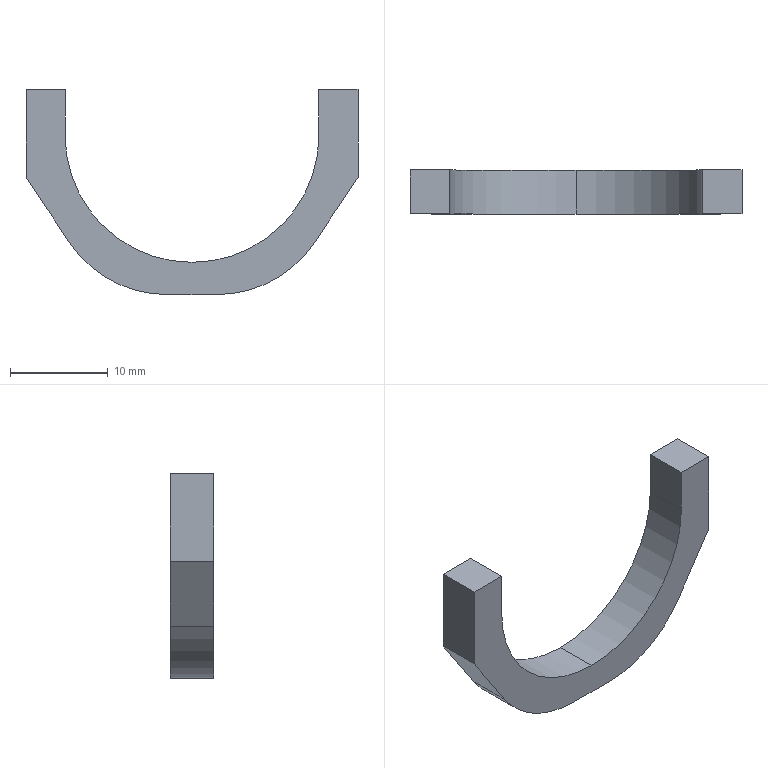Part | SolidWorks | features FlatPattern 1, SMBaseFlange 1, SheetMetal 1 | 1 solid | 15 faces | box 34 x 4.5 x 21 mm | volume 979.762 mm3 | plane 11 | cylinder 4 | commonest cylinder face diameters 24 x2 26 x2
STEP:
#1=CARTESIAN_POINT('',(0.,4.5,3.3));
#2=VERTEX_POINT('',#1);
#3=CARTESIAN_POINT('',(13.,4.5,16.3));
#4=VERTEX_POINT('',#3);
#5=CARTESIAN_POINT('',(0.,4.5,16.3));
#6=DIRECTION('',(0.,-1.,0.));
#7=DIRECTION('',(0.,0.,1.));
#8=AXIS2_PLACEMENT_3D('',#5,#6,#7);
#9=CIRCLE('',#8,13.);
#10=EDGE_CURVE('',#2,#4,#9,.T.);
#11=ORIENTED_EDGE('',*,*,#10,.F.);
#12=CARTESIAN_POINT('',(0.,0.,3.3));
#13=VERTEX_POINT('',#12);
#14=CARTESIAN_POINT('',(0.,4.5,3.3));
#15=DIRECTION('',(0.,-1.,0.));
#16=VECTOR('',#15,1000.);
#17=LINE('',#14,#16);
#18=EDGE_CURVE('',#2,#13,#17,.T.);
#19=ORIENTED_EDGE('',*,*,#18,.T.);
#20=CARTESIAN_POINT('',(13.,0.,16.3));
#21=VERTEX_POINT('',#20);
#22=CARTESIAN_POINT('',(0.,0.,16.3));
#23=DIRECTION('',(0.,-1.,0.));
#24=DIRECTION('',(0.,0.,1.));
#25=AXIS2_PLACEMENT_3D('',#22,#23,#24);
#26=CIRCLE('',#25,13.);
#27=EDGE_CURVE('',#13,#21,#26,.T.);
#28=ORIENTED_EDGE('',*,*,#27,.T.);
#29=CARTESIAN_POINT('',(13.,4.5,16.3));
#30=DIRECTION('',(0.,-1.,0.));
#31=VECTOR('',#30,1000.);
#32=LINE('',#29,#31);
#33=EDGE_CURVE('',#4,#21,#32,.T.);
#34=ORIENTED_EDGE('',*,*,#33,.F.);
#35=EDGE_LOOP('',(#11,#19,#28,#34));
#36=FACE_OUTER_BOUND('',#35,.T.);
#37=CARTESIAN_POINT('',(0.,4.5,16.3));
#38=DIRECTION('',(0.,-1.,0.));
#39=DIRECTION('',(0.,0.,-1.));
#40=AXIS2_PLACEMENT_3D('',#37,#38,#39);
#41=CYLINDRICAL_SURFACE('',#40,13.);
#42=ADVANCED_FACE('',(#36),#41,.F.);
#43=CARTESIAN_POINT('',(-12.562,0.,5.344));
#44=VERTEX_POINT('',#43);
#45=CARTESIAN_POINT('',(-17.,0.,12.));
#46=VERTEX_POINT('',#45);
#47=CARTESIAN_POINT('',(-12.562,0.,5.344));
#48=DIRECTION('',(-0.5547,0.,0.8321));
#49=VECTOR('',#48,1000.);
#50=LINE('',#47,#49);
#51=EDGE_CURVE('',#44,#46,#50,.T.);
#52=ORIENTED_EDGE('',*,*,#51,.T.);
#53=CARTESIAN_POINT('',(-17.,4.5,12.));
#54=VERTEX_POINT('',#53);
#55=CARTESIAN_POINT('',(-17.,4.5,12.));
#56=DIRECTION('',(0.,-1.,0.));
#57=VECTOR('',#56,1000.);
#58=LINE('',#55,#57);
#59=EDGE_CURVE('',#54,#46,#58,.T.);
#60=ORIENTED_EDGE('',*,*,#59,.F.);
#61=CARTESIAN_POINT('',(-12.562,4.5,5.344));
#62=VERTEX_POINT('',#61);
#63=CARTESIAN_POINT('',(-12.562,4.5,5.344));
#64=DIRECTION('',(-0.5547,0.,0.8321));
#65=VECTOR('',#64,1000.);
#66=LINE('',#63,#65);
#67=EDGE_CURVE('',#62,#54,#66,.T.);
#68=ORIENTED_EDGE('',*,*,#67,.F.);
#69=CARTESIAN_POINT('',(-12.562,4.5,5.344));
#70=DIRECTION('',(0.,-1.,0.));
#71=VECTOR('',#70,1000.);
#72=LINE('',#69,#71);
#73=EDGE_CURVE('',#62,#44,#72,.T.);
#74=ORIENTED_EDGE('',*,*,#73,.T.);
#75=EDGE_LOOP('',(#52,#60,#68,#74));
#76=FACE_OUTER_BOUND('',#75,.T.);
#77=CARTESIAN_POINT('',(-12.562,4.5,5.344));
#78=DIRECTION('',(0.8321,0.,0.5547));
#79=DIRECTION('',(0.5547,0.,-0.8321));
#80=AXIS2_PLACEMENT_3D('',#77,#78,#79);
#81=PLANE('',#80);
#82=ADVANCED_FACE('',(#76),#81,.F.);
#83=CARTESIAN_POINT('',(-17.,0.,21.));
#84=VERTEX_POINT('',#83);
#85=CARTESIAN_POINT('',(-17.,0.,12.));
#86=DIRECTION('',(0.,0.,1.));
#87=VECTOR('',#86,1000.);
#88=LINE('',#85,#87);
#89=EDGE_CURVE('',#46,#84,#88,.T.);
#90=ORIENTED_EDGE('',*,*,#89,.T.);
#91=CARTESIAN_POINT('',(-17.,4.5,21.));
#92=VERTEX_POINT('',#91);
#93=CARTESIAN_POINT('',(-17.,4.5,21.));
#94=DIRECTION('',(0.,-1.,0.));
#95=VECTOR('',#94,1000.);
#96=LINE('',#93,#95);
#97=EDGE_CURVE('',#92,#84,#96,.T.);
#98=ORIENTED_EDGE('',*,*,#97,.F.);
#99=CARTESIAN_POINT('',(-17.,4.5,12.));
#100=DIRECTION('',(0.,0.,1.));
#101=VECTOR('',#100,1000.);
#102=LINE('',#99,#101);
#103=EDGE_CURVE('',#54,#92,#102,.T.);
#104=ORIENTED_EDGE('',*,*,#103,.F.);
#105=ORIENTED_EDGE('',*,*,#59,.T.);
#106=EDGE_LOOP('',(#90,#98,#104,#105));
#107=FACE_OUTER_BOUND('',#106,.T.);
#108=CARTESIAN_POINT('',(-17.,4.5,12.));
#109=DIRECTION('',(1.,0.,0.));
#110=DIRECTION('',(0.,0.,-1.));
#111=AXIS2_PLACEMENT_3D('',#108,#109,#110);
#112=PLANE('',#111);
#113=ADVANCED_FACE('',(#107),#112,.F.);
#114=CARTESIAN_POINT('',(-13.,0.,21.));
#115=VERTEX_POINT('',#114);
#116=CARTESIAN_POINT('',(-13.,0.,21.));
#117=DIRECTION('',(1.,0.,0.));
#118=VECTOR('',#117,1000.);
#119=LINE('',#116,#118);
#120=EDGE_CURVE('',#84,#115,#119,.T.);
#121=ORIENTED_EDGE('',*,*,#120,.T.);
#122=CARTESIAN_POINT('',(-13.,4.5,21.));
#123=VERTEX_POINT('',#122);
#124=CARTESIAN_POINT('',(-13.,4.5,21.));
#125=DIRECTION('',(0.,-1.,0.));
#126=VECTOR('',#125,1000.);
#127=LINE('',#124,#126);
#128=EDGE_CURVE('',#123,#115,#127,.T.);
#129=ORIENTED_EDGE('',*,*,#128,.F.);
#130=CARTESIAN_POINT('',(-13.,4.5,21.));
#131=DIRECTION('',(1.,0.,0.));
#132=VECTOR('',#131,1000.);
#133=LINE('',#130,#132);
#134=EDGE_CURVE('',#92,#123,#133,.T.);
#135=ORIENTED_EDGE('',*,*,#134,.F.);
#136=ORIENTED_EDGE('',*,*,#97,.T.);
#137=EDGE_LOOP('',(#121,#129,#135,#136));
#138=FACE_OUTER_BOUND('',#137,.T.);
#139=CARTESIAN_POINT('',(-13.,4.5,21.));
#140=DIRECTION('',(0.,0.,-1.));
#141=DIRECTION('',(-1.,0.,0.));
#142=AXIS2_PLACEMENT_3D('',#139,#140,#141);
#143=PLANE('',#142);
#144=ADVANCED_FACE('',(#138),#143,.F.);
#145=CARTESIAN_POINT('',(-13.,0.,16.3));
#146=VERTEX_POINT('',#145);
#147=CARTESIAN_POINT('',(-13.,0.,16.3));
#148=DIRECTION('',(0.,0.,-1.));
#149=VECTOR('',#148,1000.);
#150=LINE('',#147,#149);
#151=EDGE_CURVE('',#115,#146,#150,.T.);
#152=ORIENTED_EDGE('',*,*,#151,.T.);
#153=CARTESIAN_POINT('',(-13.,4.5,16.3));
#154=VERTEX_POINT('',#153);
#155=CARTESIAN_POINT('',(-13.,4.5,16.3));
#156=DIRECTION('',(0.,-1.,0.));
#157=VECTOR('',#156,1000.);
#158=LINE('',#155,#157);
#159=EDGE_CURVE('',#154,#146,#158,.T.);
#160=ORIENTED_EDGE('',*,*,#159,.F.);
#161=CARTESIAN_POINT('',(-13.,4.5,16.3));
#162=DIRECTION('',(0.,0.,-1.));
#163=VECTOR('',#162,1000.);
#164=LINE('',#161,#163);
#165=EDGE_CURVE('',#123,#154,#164,.T.);
#166=ORIENTED_EDGE('',*,*,#165,.F.);
#167=ORIENTED_EDGE('',*,*,#128,.T.);
#168=EDGE_LOOP('',(#152,#160,#166,#167));
#169=FACE_OUTER_BOUND('',#168,.T.);
#170=CARTESIAN_POINT('',(-13.,4.5,16.3));
#171=DIRECTION('',(-1.,0.,0.));
#172=DIRECTION('',(0.,0.,1.));
#173=AXIS2_PLACEMENT_3D('',#170,#171,#172);
#174=PLANE('',#173);
#175=ADVANCED_FACE('',(#169),#174,.F.);
#176=ORIENTED_EDGE('',*,*,#18,.F.);
#177=CARTESIAN_POINT('',(0.,4.5,16.3));
#178=DIRECTION('',(0.,-1.,0.));
#179=DIRECTION('',(0.,0.,1.));
#180=AXIS2_PLACEMENT_3D('',#177,#178,#179);
#181=CIRCLE('',#180,13.);
#182=EDGE_CURVE('',#154,#2,#181,.T.);
#183=ORIENTED_EDGE('',*,*,#182,.F.);
#184=ORIENTED_EDGE('',*,*,#159,.T.);
#185=CARTESIAN_POINT('',(0.,0.,16.3));
#186=DIRECTION('',(0.,-1.,0.));
#187=DIRECTION('',(0.,0.,1.));
#188=AXIS2_PLACEMENT_3D('',#185,#186,#187);
#189=CIRCLE('',#188,13.);
#190=EDGE_CURVE('',#146,#13,#189,.T.);
#191=ORIENTED_EDGE('',*,*,#190,.T.);
#192=EDGE_LOOP('',(#176,#183,#184,#191));
#193=FACE_OUTER_BOUND('',#192,.T.);
#194=CARTESIAN_POINT('',(0.,4.5,16.3));
#195=DIRECTION('',(0.,-1.,0.));
#196=DIRECTION('',(0.,0.,-1.));
#197=AXIS2_PLACEMENT_3D('',#194,#195,#196);
#198=CYLINDRICAL_SURFACE('',#197,13.);
#199=ADVANCED_FACE('',(#193),#198,.F.);
#200=CARTESIAN_POINT('',(13.,0.,21.));
#201=VERTEX_POINT('',#200);
#202=CARTESIAN_POINT('',(13.,0.,16.3));
#203=DIRECTION('',(0.,0.,1.));
#204=VECTOR('',#203,1000.);
#205=LINE('',#202,#204);
#206=EDGE_CURVE('',#21,#201,#205,.T.);
#207=ORIENTED_EDGE('',*,*,#206,.T.);
#208=CARTESIAN_POINT('',(13.,4.5,21.));
#209=VERTEX_POINT('',#208);
#210=CARTESIAN_POINT('',(13.,4.5,21.));
#211=DIRECTION('',(0.,-1.,0.));
#212=VECTOR('',#211,1000.);
#213=LINE('',#210,#212);
#214=EDGE_CURVE('',#209,#201,#213,.T.);
#215=ORIENTED_EDGE('',*,*,#214,.F.);
#216=CARTESIAN_POINT('',(13.,4.5,16.3));
#217=DIRECTION('',(0.,0.,1.));
#218=VECTOR('',#217,1000.);
#219=LINE('',#216,#218);
#220=EDGE_CURVE('',#4,#209,#219,.T.);
#221=ORIENTED_EDGE('',*,*,#220,.F.);
#222=ORIENTED_EDGE('',*,*,#33,.T.);
#223=EDGE_LOOP('',(#207,#215,#221,#222));
#224=FACE_OUTER_BOUND('',#223,.T.);
#225=CARTESIAN_POINT('',(13.,4.5,16.3));
#226=DIRECTION('',(1.,0.,0.));
#227=DIRECTION('',(0.,0.,-1.));
#228=AXIS2_PLACEMENT_3D('',#225,#226,#227);
#229=PLANE('',#228);
#230=ADVANCED_FACE('',(#224),#229,.F.);
#231=CARTESIAN_POINT('',(17.,0.,21.));
#232=VERTEX_POINT('',#231);
#233=CARTESIAN_POINT('',(13.,0.,21.));
#234=DIRECTION('',(1.,0.,0.));
#235=VECTOR('',#234,1000.);
#236=LINE('',#233,#235);
#237=EDGE_CURVE('',#201,#232,#236,.T.);
#238=ORIENTED_EDGE('',*,*,#237,.T.);
#239=CARTESIAN_POINT('',(17.,4.5,21.));
#240=VERTEX_POINT('',#239);
#241=CARTESIAN_POINT('',(17.,4.5,21.));
#242=DIRECTION('',(0.,-1.,0.));
#243=VECTOR('',#242,1000.);
#244=LINE('',#241,#243);
#245=EDGE_CURVE('',#240,#232,#244,.T.);
#246=ORIENTED_EDGE('',*,*,#245,.F.);
#247=CARTESIAN_POINT('',(13.,4.5,21.));
#248=DIRECTION('',(1.,0.,0.));
#249=VECTOR('',#248,1000.);
#250=LINE('',#247,#249);
#251=EDGE_CURVE('',#209,#240,#250,.T.);
#252=ORIENTED_EDGE('',*,*,#251,.F.);
#253=ORIENTED_EDGE('',*,*,#214,.T.);
#254=EDGE_LOOP('',(#238,#246,#252,#253));
#255=FACE_OUTER_BOUND('',#254,.T.);
#256=CARTESIAN_POINT('',(13.,4.5,21.));
#257=DIRECTION('',(0.,0.,-1.));
#258=DIRECTION('',(-1.,0.,0.));
#259=AXIS2_PLACEMENT_3D('',#256,#257,#258);
#260=PLANE('',#259);
#261=ADVANCED_FACE('',(#255),#260,.F.);
#262=CARTESIAN_POINT('',(17.,0.,12.));
#263=VERTEX_POINT('',#262);
#264=CARTESIAN_POINT('',(17.,0.,12.));
#265=DIRECTION('',(0.,0.,-1.));
#266=VECTOR('',#265,1000.);
#267=LINE('',#264,#266);
#268=EDGE_CURVE('',#232,#263,#267,.T.);
#269=ORIENTED_EDGE('',*,*,#268,.T.);
#270=CARTESIAN_POINT('',(17.,4.5,12.));
#271=VERTEX_POINT('',#270);
#272=CARTESIAN_POINT('',(17.,4.5,12.));
#273=DIRECTION('',(0.,-1.,0.));
#274=VECTOR('',#273,1000.);
#275=LINE('',#272,#274);
#276=EDGE_CURVE('',#271,#263,#275,.T.);
#277=ORIENTED_EDGE('',*,*,#276,.F.);
#278=CARTESIAN_POINT('',(17.,4.5,12.));
#279=DIRECTION('',(0.,0.,-1.));
#280=VECTOR('',#279,1000.);
#281=LINE('',#278,#280);
#282=EDGE_CURVE('',#240,#271,#281,.T.);
#283=ORIENTED_EDGE('',*,*,#282,.F.);
#284=ORIENTED_EDGE('',*,*,#245,.T.);
#285=EDGE_LOOP('',(#269,#277,#283,#284));
#286=FACE_OUTER_BOUND('',#285,.T.);
#287=CARTESIAN_POINT('',(17.,4.5,12.));
#288=DIRECTION('',(-1.,0.,0.));
#289=DIRECTION('',(0.,0.,1.));
#290=AXIS2_PLACEMENT_3D('',#287,#288,#289);
#291=PLANE('',#290);
#292=ADVANCED_FACE('',(#286),#291,.F.);
#293=CARTESIAN_POINT('',(12.562,0.,5.344));
#294=VERTEX_POINT('',#293);
#295=CARTESIAN_POINT('',(12.562,0.,5.344));
#296=DIRECTION('',(-0.5547,0.,-0.8321));
#297=VECTOR('',#296,1000.);
#298=LINE('',#295,#297);
#299=EDGE_CURVE('',#263,#294,#298,.T.);
#300=ORIENTED_EDGE('',*,*,#299,.T.);
#301=CARTESIAN_POINT('',(12.562,4.5,5.344));
#302=VERTEX_POINT('',#301);
#303=CARTESIAN_POINT('',(12.562,4.5,5.344));
#304=DIRECTION('',(0.,-1.,0.));
#305=VECTOR('',#304,1000.);
#306=LINE('',#303,#305);
#307=EDGE_CURVE('',#302,#294,#306,.T.);
#308=ORIENTED_EDGE('',*,*,#307,.F.);
#309=CARTESIAN_POINT('',(12.562,4.5,5.344));
#310=DIRECTION('',(-0.5547,0.,-0.8321));
#311=VECTOR('',#310,1000.);
#312=LINE('',#309,#311);
#313=EDGE_CURVE('',#271,#302,#312,.T.);
#314=ORIENTED_EDGE('',*,*,#313,.F.);
#315=ORIENTED_EDGE('',*,*,#276,.T.);
#316=EDGE_LOOP('',(#300,#308,#314,#315));
#317=FACE_OUTER_BOUND('',#316,.T.);
#318=CARTESIAN_POINT('',(12.562,4.5,5.344));
#319=DIRECTION('',(-0.8321,0.,0.5547));
#320=DIRECTION('',(0.5547,0.,0.8321));
#321=AXIS2_PLACEMENT_3D('',#318,#319,#320);
#322=PLANE('',#321);
#323=ADVANCED_FACE('',(#317),#322,.F.);
#324=CARTESIAN_POINT('',(2.578,0.,0.));
#325=VERTEX_POINT('',#324);
#326=CARTESIAN_POINT('',(2.578,0.,12.));
#327=DIRECTION('',(0.,1.,0.));
#328=DIRECTION('',(0.,0.,-1.));
#329=AXIS2_PLACEMENT_3D('',#326,#327,#328);
#330=CIRCLE('',#329,12.);
#331=EDGE_CURVE('',#294,#325,#330,.T.);
#332=ORIENTED_EDGE('',*,*,#331,.T.);
#333=CARTESIAN_POINT('',(2.578,4.5,0.));
#334=VERTEX_POINT('',#333);
#335=CARTESIAN_POINT('',(2.578,4.5,0.));
#336=DIRECTION('',(0.,-1.,0.));
#337=VECTOR('',#336,1000.);
#338=LINE('',#335,#337);
#339=EDGE_CURVE('',#334,#325,#338,.T.);
#340=ORIENTED_EDGE('',*,*,#339,.F.);
#341=CARTESIAN_POINT('',(2.578,4.5,12.));
#342=DIRECTION('',(0.,1.,0.));
#343=DIRECTION('',(0.,0.,-1.));
#344=AXIS2_PLACEMENT_3D('',#341,#342,#343);
#345=CIRCLE('',#344,12.);
#346=EDGE_CURVE('',#302,#334,#345,.T.);
#347=ORIENTED_EDGE('',*,*,#346,.F.);
#348=ORIENTED_EDGE('',*,*,#307,.T.);
#349=EDGE_LOOP('',(#332,#340,#347,#348));
#350=FACE_OUTER_BOUND('',#349,.T.);
#351=CARTESIAN_POINT('',(2.578,4.5,12.));
#352=DIRECTION('',(0.,-1.,0.));
#353=DIRECTION('',(0.,0.,-1.));
#354=AXIS2_PLACEMENT_3D('',#351,#352,#353);
#355=CYLINDRICAL_SURFACE('',#354,12.);
#356=ADVANCED_FACE('',(#350),#355,.T.);
#357=CARTESIAN_POINT('',(-2.578,0.,0.));
#358=VERTEX_POINT('',#357);
#359=CARTESIAN_POINT('',(-2.578,0.,0.));
#360=DIRECTION('',(-1.,0.,0.));
#361=VECTOR('',#360,1000.);
#362=LINE('',#359,#361);
#363=EDGE_CURVE('',#325,#358,#362,.T.);
#364=ORIENTED_EDGE('',*,*,#363,.T.);
#365=CARTESIAN_POINT('',(-2.578,4.5,0.));
#366=VERTEX_POINT('',#365);
#367=CARTESIAN_POINT('',(-2.578,4.5,0.));
#368=DIRECTION('',(0.,-1.,0.));
#369=VECTOR('',#368,1000.);
#370=LINE('',#367,#369);
#371=EDGE_CURVE('',#366,#358,#370,.T.);
#372=ORIENTED_EDGE('',*,*,#371,.F.);
#373=CARTESIAN_POINT('',(-2.578,4.5,0.));
#374=DIRECTION('',(-1.,0.,0.));
#375=VECTOR('',#374,1000.);
#376=LINE('',#373,#375);
#377=EDGE_CURVE('',#334,#366,#376,.T.);
#378=ORIENTED_EDGE('',*,*,#377,.F.);
#379=ORIENTED_EDGE('',*,*,#339,.T.);
#380=EDGE_LOOP('',(#364,#372,#378,#379));
#381=FACE_OUTER_BOUND('',#380,.T.);
#382=CARTESIAN_POINT('',(-2.578,4.5,0.));
#383=DIRECTION('',(0.,0.,1.));
#384=DIRECTION('',(1.,0.,0.));
#385=AXIS2_PLACEMENT_3D('',#382,#383,#384);
#386=PLANE('',#385);
#387=ADVANCED_FACE('',(#381),#386,.F.);
#388=CARTESIAN_POINT('',(-2.578,0.,12.));
#389=DIRECTION('',(0.,1.,0.));
#390=DIRECTION('',(0.,0.,-1.));
#391=AXIS2_PLACEMENT_3D('',#388,#389,#390);
#392=CIRCLE('',#391,12.);
#393=EDGE_CURVE('',#358,#44,#392,.T.);
#394=ORIENTED_EDGE('',*,*,#393,.T.);
#395=ORIENTED_EDGE('',*,*,#73,.F.);
#396=CARTESIAN_POINT('',(-2.578,4.5,12.));
#397=DIRECTION('',(0.,1.,0.));
#398=DIRECTION('',(0.,0.,-1.));
#399=AXIS2_PLACEMENT_3D('',#396,#397,#398);
#400=CIRCLE('',#399,12.);
#401=EDGE_CURVE('',#366,#62,#400,.T.);
#402=ORIENTED_EDGE('',*,*,#401,.F.);
#403=ORIENTED_EDGE('',*,*,#371,.T.);
#404=EDGE_LOOP('',(#394,#395,#402,#403));
#405=FACE_OUTER_BOUND('',#404,.T.);
#406=CARTESIAN_POINT('',(-2.578,4.5,12.));
#407=DIRECTION('',(0.,-1.,0.));
#408=DIRECTION('',(0.,0.,-1.));
#409=AXIS2_PLACEMENT_3D('',#406,#407,#408);
#410=CYLINDRICAL_SURFACE('',#409,12.);
#411=ADVANCED_FACE('',(#405),#410,.T.);
#412=ORIENTED_EDGE('',*,*,#67,.T.);
#413=ORIENTED_EDGE('',*,*,#103,.T.);
#414=ORIENTED_EDGE('',*,*,#134,.T.);
#415=ORIENTED_EDGE('',*,*,#165,.T.);
#416=ORIENTED_EDGE('',*,*,#182,.T.);
#417=ORIENTED_EDGE('',*,*,#10,.T.);
#418=ORIENTED_EDGE('',*,*,#220,.T.);
#419=ORIENTED_EDGE('',*,*,#251,.T.);
#420=ORIENTED_EDGE('',*,*,#282,.T.);
#421=ORIENTED_EDGE('',*,*,#313,.T.);
#422=ORIENTED_EDGE('',*,*,#346,.T.);
#423=ORIENTED_EDGE('',*,*,#377,.T.);
#424=ORIENTED_EDGE('',*,*,#401,.T.);
#425=EDGE_LOOP('',(#412,#413,#414,#415,#416,#417,#418,#419,#420,#421,#422,#423,#424));
#426=FACE_OUTER_BOUND('',#425,.T.);
#427=CARTESIAN_POINT('',(0.,4.5,16.3));
#428=DIRECTION('',(0.,1.,0.));
#429=DIRECTION('',(0.,0.,1.));
#430=AXIS2_PLACEMENT_3D('',#427,#428,#429);
#431=PLANE('',#430);
#432=ADVANCED_FACE('',(#426),#431,.T.);
#433=ORIENTED_EDGE('',*,*,#51,.F.);
#434=ORIENTED_EDGE('',*,*,#393,.F.);
#435=ORIENTED_EDGE('',*,*,#363,.F.);
#436=ORIENTED_EDGE('',*,*,#331,.F.);
#437=ORIENTED_EDGE('',*,*,#299,.F.);
#438=ORIENTED_EDGE('',*,*,#268,.F.);
#439=ORIENTED_EDGE('',*,*,#237,.F.);
#440=ORIENTED_EDGE('',*,*,#206,.F.);
#441=ORIENTED_EDGE('',*,*,#27,.F.);
#442=ORIENTED_EDGE('',*,*,#190,.F.);
#443=ORIENTED_EDGE('',*,*,#151,.F.);
#444=ORIENTED_EDGE('',*,*,#120,.F.);
#445=ORIENTED_EDGE('',*,*,#89,.F.);
#446=EDGE_LOOP('',(#433,#434,#435,#436,#437,#438,#439,#440,#441,#442,#443,#444,#445));
#447=FACE_OUTER_BOUND('',#446,.T.);
#448=CARTESIAN_POINT('',(0.,0.,16.3));
#449=DIRECTION('',(0.,1.,0.));
#450=DIRECTION('',(0.,0.,1.));
#451=AXIS2_PLACEMENT_3D('',#448,#449,#450);
#452=PLANE('',#451);
#453=ADVANCED_FACE('',(#447),#452,.F.);
#454=CLOSED_SHELL('',(#42,#82,#113,#144,#175,#199,#230,#261,#292,#323,#356,#387,#411,#432,#453));
#455=MANIFOLD_SOLID_BREP('',#454);
#456=CARTESIAN_POINT('',(0.,0.,0.));
#457=DIRECTION('',(0.,0.,1.));
#458=DIRECTION('',(1.,0.,0.));
#459=AXIS2_PLACEMENT_3D('',#456,#457,#458);
#460=(LENGTH_UNIT()NAMED_UNIT(*)SI_UNIT(.MILLI.,.METRE.));
#461=UNCERTAINTY_MEASURE_WITH_UNIT(LENGTH_MEASURE(0.00001),#460,'','');
#462=(NAMED_UNIT(*)PLANE_ANGLE_UNIT()SI_UNIT($,.RADIAN.));
#463=(NAMED_UNIT(*)SI_UNIT($,.STERADIAN.)SOLID_ANGLE_UNIT());
#464=(GEOMETRIC_REPRESENTATION_CONTEXT(3)GLOBAL_UNCERTAINTY_ASSIGNED_CONTEXT((#461))GLOBAL_UNIT_ASSIGNED_CONTEXT((#460,#462,#463))REPRESENTATION_CONTEXT('',''));
#465=ADVANCED_BREP_SHAPE_REPRESENTATION('',(#455,#459),#464);